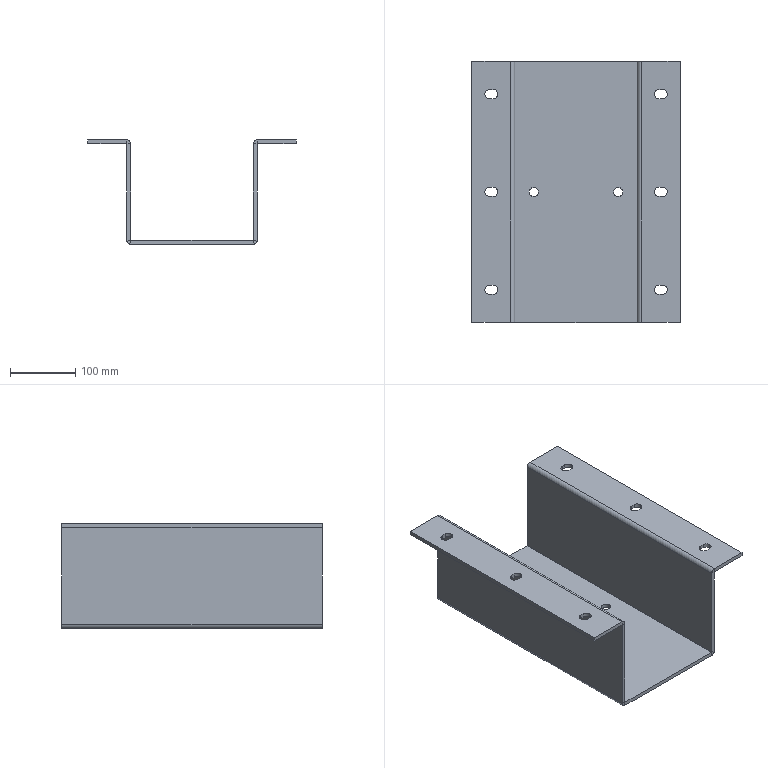Part | 1 solid | 72 faces | box 320 x 400 x 160 mm | volume 1483602 mm3 | plane 42 | cylinder 30 | commonest cylinder face diameters 14 x22 0.4 x4 12.4 x4